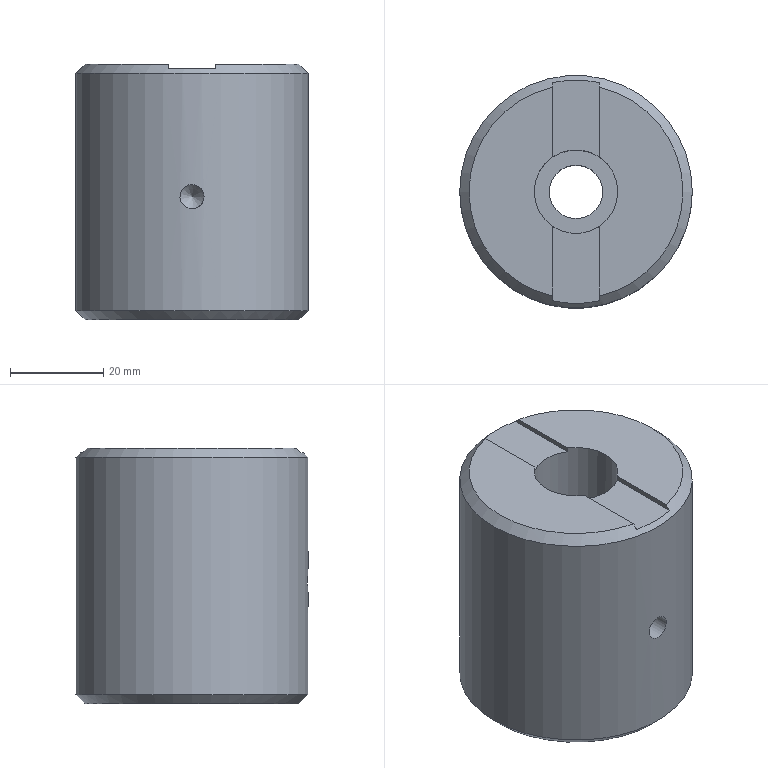Part | NX | features LIN_SOLID_COLOR 2 | 1 solid | 17 faces | box 50 x 50 x 55 mm | volume 97336 mm3 | plane 10 | cylinder 4 | cone 3 | commonest cylinder face diameters 5.2 x1 11.5 x1 18 x1 50 x1
STEP:
#1=CARTESIAN_POINT('',(609.,-200.,-46.5));
#2=VERTEX_POINT('',#1);
#3=CARTESIAN_POINT('',(586.,-200.,-46.5));
#4=DIRECTION('',(0.,0.,1.));
#5=DIRECTION('',(1.,0.,0.));
#6=AXIS2_PLACEMENT_3D('',#3,#4,#5);
#7=CIRCLE('',#6,23.);
#8=EDGE_CURVE('',#2,#2,#7,.T.);
#9=ORIENTED_EDGE('',*,*,#8,.F.);
#10=EDGE_LOOP('',(#9));
#11=FACE_BOUND('',#10,.T.);
#12=CARTESIAN_POINT('',(591.75,-200.,-46.5));
#13=VERTEX_POINT('',#12);
#14=CARTESIAN_POINT('',(586.,-200.,-46.5));
#15=DIRECTION('',(0.,0.,1.));
#16=DIRECTION('',(1.,0.,0.));
#17=AXIS2_PLACEMENT_3D('',#14,#15,#16);
#18=CIRCLE('',#17,5.75);
#19=EDGE_CURVE('',#13,#13,#18,.T.);
#20=ORIENTED_EDGE('',*,*,#19,.T.);
#21=EDGE_LOOP('',(#20));
#22=FACE_BOUND('',#21,.T.);
#23=CARTESIAN_POINT('',(586.,-200.,-46.5));
#24=DIRECTION('',(0.,0.,-1.));
#25=DIRECTION('',(1.,0.,0.));
#26=AXIS2_PLACEMENT_3D('',#23,#24,#25);
#27=PLANE('',#26);
#28=ADVANCED_FACE('',(#11,#22),#27,.T.);
#29=CARTESIAN_POINT('',(591.,-177.55,8.5));
#30=VERTEX_POINT('',#29);
#31=CARTESIAN_POINT('',(591.,-192.517,8.5));
#32=VERTEX_POINT('',#31);
#33=CARTESIAN_POINT('',(591.,-200.,8.5));
#34=DIRECTION('',(0.,-1.,0.));
#35=VECTOR('',#34,1000.);
#36=LINE('',#33,#35);
#37=EDGE_CURVE('',#30,#32,#36,.T.);
#38=ORIENTED_EDGE('',*,*,#37,.T.);
#39=CARTESIAN_POINT('',(591.,-207.483,8.5));
#40=VERTEX_POINT('',#39);
#41=CARTESIAN_POINT('',(586.,-200.,8.5));
#42=DIRECTION('',(0.,0.,-1.));
#43=DIRECTION('',(1.,0.,0.));
#44=AXIS2_PLACEMENT_3D('',#41,#42,#43);
#45=CIRCLE('',#44,9.);
#46=EDGE_CURVE('',#32,#40,#45,.T.);
#47=ORIENTED_EDGE('',*,*,#46,.T.);
#48=CARTESIAN_POINT('',(591.,-222.45,8.5));
#49=VERTEX_POINT('',#48);
#50=CARTESIAN_POINT('',(591.,-200.,8.5));
#51=DIRECTION('',(0.,-1.,0.));
#52=VECTOR('',#51,1000.);
#53=LINE('',#50,#52);
#54=EDGE_CURVE('',#40,#49,#53,.T.);
#55=ORIENTED_EDGE('',*,*,#54,.T.);
#56=CARTESIAN_POINT('',(586.,-200.,8.5));
#57=DIRECTION('',(0.,0.,-1.));
#58=DIRECTION('',(-1.,0.,0.));
#59=AXIS2_PLACEMENT_3D('',#56,#57,#58);
#60=CIRCLE('',#59,23.);
#61=EDGE_CURVE('',#30,#49,#60,.T.);
#62=ORIENTED_EDGE('',*,*,#61,.F.);
#63=EDGE_LOOP('',(#38,#47,#55,#62));
#64=FACE_BOUND('',#63,.T.);
#65=CARTESIAN_POINT('',(586.,-200.,8.5));
#66=DIRECTION('',(0.,0.,1.));
#67=DIRECTION('',(-1.,0.,0.));
#68=AXIS2_PLACEMENT_3D('',#65,#66,#67);
#69=PLANE('',#68);
#70=ADVANCED_FACE('',(#64),#69,.T.);
#71=CARTESIAN_POINT('',(581.,-222.45,8.5));
#72=VERTEX_POINT('',#71);
#73=CARTESIAN_POINT('',(581.,-207.483,8.5));
#74=VERTEX_POINT('',#73);
#75=CARTESIAN_POINT('',(581.,-200.,8.5));
#76=DIRECTION('',(0.,1.,0.));
#77=VECTOR('',#76,1000.);
#78=LINE('',#75,#77);
#79=EDGE_CURVE('',#72,#74,#78,.T.);
#80=ORIENTED_EDGE('',*,*,#79,.T.);
#81=CARTESIAN_POINT('',(581.,-192.517,8.5));
#82=VERTEX_POINT('',#81);
#83=CARTESIAN_POINT('',(586.,-200.,8.5));
#84=DIRECTION('',(0.,0.,-1.));
#85=DIRECTION('',(1.,0.,0.));
#86=AXIS2_PLACEMENT_3D('',#83,#84,#85);
#87=CIRCLE('',#86,9.);
#88=EDGE_CURVE('',#74,#82,#87,.T.);
#89=ORIENTED_EDGE('',*,*,#88,.T.);
#90=CARTESIAN_POINT('',(581.,-177.55,8.5));
#91=VERTEX_POINT('',#90);
#92=CARTESIAN_POINT('',(581.,-200.,8.5));
#93=DIRECTION('',(0.,1.,0.));
#94=VECTOR('',#93,1000.);
#95=LINE('',#92,#94);
#96=EDGE_CURVE('',#82,#91,#95,.T.);
#97=ORIENTED_EDGE('',*,*,#96,.T.);
#98=CARTESIAN_POINT('',(586.,-200.,8.5));
#99=DIRECTION('',(0.,0.,-1.));
#100=DIRECTION('',(-1.,0.,0.));
#101=AXIS2_PLACEMENT_3D('',#98,#99,#100);
#102=CIRCLE('',#101,23.);
#103=EDGE_CURVE('',#72,#91,#102,.T.);
#104=ORIENTED_EDGE('',*,*,#103,.F.);
#105=EDGE_LOOP('',(#80,#89,#97,#104));
#106=FACE_BOUND('',#105,.T.);
#107=CARTESIAN_POINT('',(586.,-200.,8.5));
#108=DIRECTION('',(0.,0.,1.));
#109=DIRECTION('',(-1.,0.,0.));
#110=AXIS2_PLACEMENT_3D('',#107,#108,#109);
#111=PLANE('',#110);
#112=ADVANCED_FACE('',(#106),#111,.T.);
#113=CARTESIAN_POINT('',(588.6,-224.864,-20.));
#114=VERTEX_POINT('',#113);
#115=CARTESIAN_POINT('',(588.036,-224.933,-22.04));
#116=CARTESIAN_POINT('',(588.882,-224.83,-19.999));
#117=CARTESIAN_POINT('',(588.036,-224.932,-17.962));
#118=CARTESIAN_POINT('',(586.002,-225.034,-17.119));
#119=CARTESIAN_POINT('',(583.963,-224.932,-17.961));
#120=CARTESIAN_POINT('',(583.119,-224.83,-19.999));
#121=CARTESIAN_POINT('',(583.961,-224.932,-22.035));
#122=CARTESIAN_POINT('',(585.997,-225.034,-22.881));
#123=CARTESIAN_POINT('',(588.036,-224.933,-22.04));
#124=CARTESIAN_POINT('',(588.882,-224.83,-19.999));
#125=CARTESIAN_POINT('',(588.036,-224.932,-17.962));
#126=B_SPLINE_CURVE_WITH_KNOTS('',3,(#115,#116,#117,#118,#119,#120,#121,#122,#123,#124,#125),.UNSPECIFIED.,.T.,.F.,(1,1,1,1,1,1,1,1,1,1,1,1,1,1,1),(-0.0061,-0.004067,-0.002033,0.,0.002033,0.004067,0.0061,0.008133,0.01017,0.0122,0.01423,0.01627,0.0183,0.02033,0.02237),.UNSPECIFIED.);
#127=EDGE_CURVE('',#114,#114,#126,.T.);
#128=ORIENTED_EDGE('',*,*,#127,.F.);
#129=EDGE_LOOP('',(#128));
#130=FACE_BOUND('',#129,.T.);
#131=CARTESIAN_POINT('',(611.,-200.,-44.5));
#132=VERTEX_POINT('',#131);
#133=CARTESIAN_POINT('',(586.,-200.,-44.5));
#134=DIRECTION('',(0.,0.,1.));
#135=DIRECTION('',(1.,0.,0.));
#136=AXIS2_PLACEMENT_3D('',#133,#134,#135);
#137=CIRCLE('',#136,25.);
#138=EDGE_CURVE('',#132,#132,#137,.F.);
#139=ORIENTED_EDGE('',*,*,#138,.F.);
#140=EDGE_LOOP('',(#139));
#141=FACE_BOUND('',#140,.T.);
#142=CARTESIAN_POINT('',(561.,-200.,6.5));
#143=VERTEX_POINT('',#142);
#144=CARTESIAN_POINT('',(586.,-200.,6.5));
#145=DIRECTION('',(0.,0.,-1.));
#146=DIRECTION('',(-1.,0.,0.));
#147=AXIS2_PLACEMENT_3D('',#144,#145,#146);
#148=CIRCLE('',#147,25.);
#149=EDGE_CURVE('',#143,#143,#148,.F.);
#150=ORIENTED_EDGE('',*,*,#149,.F.);
#151=EDGE_LOOP('',(#150));
#152=FACE_BOUND('',#151,.T.);
#153=CARTESIAN_POINT('',(586.,-200.,3.5));
#154=DIRECTION('',(0.,0.,-1.));
#155=DIRECTION('',(1.,0.,0.));
#156=AXIS2_PLACEMENT_3D('',#153,#154,#155);
#157=CYLINDRICAL_SURFACE('',#156,25.);
#158=ADVANCED_FACE('',(#130,#141,#152),#157,.T.);
#159=ORIENTED_EDGE('',*,*,#138,.T.);
#160=EDGE_LOOP('',(#159));
#161=FACE_BOUND('',#160,.T.);
#162=ORIENTED_EDGE('',*,*,#8,.T.);
#163=EDGE_LOOP('',(#162));
#164=FACE_BOUND('',#163,.T.);
#165=CARTESIAN_POINT('',(586.,-200.,-46.5));
#166=DIRECTION('',(0.,0.,1.));
#167=DIRECTION('',(-1.,0.,0.));
#168=AXIS2_PLACEMENT_3D('',#165,#166,#167);
#169=CONICAL_SURFACE('',#168,23.,0.7854);
#170=ADVANCED_FACE('',(#161,#164),#169,.T.);
#171=CARTESIAN_POINT('',(591.,-223.473,7.5));
#172=VERTEX_POINT('',#171);
#173=CARTESIAN_POINT('',(591.,-222.45,8.5));
#174=CARTESIAN_POINT('',(591.,-222.791,8.167));
#175=CARTESIAN_POINT('',(591.,-223.132,7.834));
#176=CARTESIAN_POINT('',(591.,-223.473,7.5));
#177=B_SPLINE_CURVE_WITH_KNOTS('',3,(#173,#174,#175,#176),.UNSPECIFIED.,.F.,.F.,(4,4),(0.1023,0.1037),.UNSPECIFIED.);
#178=EDGE_CURVE('',#49,#172,#177,.T.);
#179=ORIENTED_EDGE('',*,*,#178,.T.);
#180=CARTESIAN_POINT('',(581.,-223.473,7.5));
#181=VERTEX_POINT('',#180);
#182=CARTESIAN_POINT('',(586.,-200.,7.5));
#183=DIRECTION('',(0.,0.,1.));
#184=DIRECTION('',(1.,0.,0.));
#185=AXIS2_PLACEMENT_3D('',#182,#183,#184);
#186=CIRCLE('',#185,24.);
#187=EDGE_CURVE('',#172,#181,#186,.F.);
#188=ORIENTED_EDGE('',*,*,#187,.T.);
#189=CARTESIAN_POINT('',(581.,-223.473,7.5));
#190=CARTESIAN_POINT('',(581.,-223.132,7.834));
#191=CARTESIAN_POINT('',(581.,-222.791,8.167));
#192=CARTESIAN_POINT('',(581.,-222.45,8.5));
#193=B_SPLINE_CURVE_WITH_KNOTS('',3,(#189,#190,#191,#192),.UNSPECIFIED.,.F.,.F.,(4,4),(0.04264,0.04407),.UNSPECIFIED.);
#194=EDGE_CURVE('',#181,#72,#193,.T.);
#195=ORIENTED_EDGE('',*,*,#194,.T.);
#196=ORIENTED_EDGE('',*,*,#103,.T.);
#197=CARTESIAN_POINT('',(581.,-176.527,7.5));
#198=VERTEX_POINT('',#197);
#199=CARTESIAN_POINT('',(581.,-177.55,8.5));
#200=CARTESIAN_POINT('',(581.,-177.209,8.167));
#201=CARTESIAN_POINT('',(581.,-176.868,7.834));
#202=CARTESIAN_POINT('',(581.,-176.527,7.5));
#203=B_SPLINE_CURVE_WITH_KNOTS('',3,(#199,#200,#201,#202),.UNSPECIFIED.,.F.,.F.,(4,4),(0.1023,0.1037),.UNSPECIFIED.);
#204=EDGE_CURVE('',#91,#198,#203,.T.);
#205=ORIENTED_EDGE('',*,*,#204,.T.);
#206=CARTESIAN_POINT('',(591.,-176.527,7.5));
#207=VERTEX_POINT('',#206);
#208=CARTESIAN_POINT('',(586.,-200.,7.5));
#209=DIRECTION('',(0.,0.,1.));
#210=DIRECTION('',(1.,0.,0.));
#211=AXIS2_PLACEMENT_3D('',#208,#209,#210);
#212=CIRCLE('',#211,24.);
#213=EDGE_CURVE('',#198,#207,#212,.F.);
#214=ORIENTED_EDGE('',*,*,#213,.T.);
#215=CARTESIAN_POINT('',(591.,-176.527,7.5));
#216=CARTESIAN_POINT('',(591.,-176.868,7.834));
#217=CARTESIAN_POINT('',(591.,-177.209,8.167));
#218=CARTESIAN_POINT('',(591.,-177.55,8.5));
#219=B_SPLINE_CURVE_WITH_KNOTS('',3,(#215,#216,#217,#218),.UNSPECIFIED.,.F.,.F.,(4,4),(0.04264,0.04407),.UNSPECIFIED.);
#220=EDGE_CURVE('',#207,#30,#219,.T.);
#221=ORIENTED_EDGE('',*,*,#220,.T.);
#222=ORIENTED_EDGE('',*,*,#61,.T.);
#223=EDGE_LOOP('',(#179,#188,#195,#196,#205,#214,#221,#222));
#224=FACE_BOUND('',#223,.T.);
#225=ORIENTED_EDGE('',*,*,#149,.T.);
#226=EDGE_LOOP('',(#225));
#227=FACE_BOUND('',#226,.T.);
#228=CARTESIAN_POINT('',(586.,-200.,6.5));
#229=DIRECTION('',(0.,0.,-1.));
#230=DIRECTION('',(1.,0.,0.));
#231=AXIS2_PLACEMENT_3D('',#228,#229,#230);
#232=CONICAL_SURFACE('',#231,25.,0.7854);
#233=ADVANCED_FACE('',(#224,#227),#232,.T.);
#234=ORIENTED_EDGE('',*,*,#96,.F.);
#235=CARTESIAN_POINT('',(581.,-192.517,7.5));
#236=VERTEX_POINT('',#235);
#237=CARTESIAN_POINT('',(581.,-192.517,8.5));
#238=DIRECTION('',(0.,0.,-1.));
#239=VECTOR('',#238,1000.);
#240=LINE('',#237,#239);
#241=EDGE_CURVE('',#82,#236,#240,.T.);
#242=ORIENTED_EDGE('',*,*,#241,.T.);
#243=CARTESIAN_POINT('',(581.,-200.,7.5));
#244=DIRECTION('',(0.,1.,0.));
#245=VECTOR('',#244,1000.);
#246=LINE('',#243,#245);
#247=EDGE_CURVE('',#198,#236,#246,.F.);
#248=ORIENTED_EDGE('',*,*,#247,.F.);
#249=ORIENTED_EDGE('',*,*,#204,.F.);
#250=EDGE_LOOP('',(#234,#242,#248,#249));
#251=FACE_BOUND('',#250,.T.);
#252=CARTESIAN_POINT('',(581.,-200.,7.5));
#253=DIRECTION('',(-1.,0.,0.));
#254=DIRECTION('',(0.,0.,-1.));
#255=AXIS2_PLACEMENT_3D('',#252,#253,#254);
#256=PLANE('',#255);
#257=ADVANCED_FACE('',(#251),#256,.F.);
#258=ORIENTED_EDGE('',*,*,#247,.T.);
#259=CARTESIAN_POINT('',(591.,-192.517,7.5));
#260=VERTEX_POINT('',#259);
#261=CARTESIAN_POINT('',(586.,-200.,7.5));
#262=DIRECTION('',(0.,0.,-1.));
#263=DIRECTION('',(-1.,0.,0.));
#264=AXIS2_PLACEMENT_3D('',#261,#262,#263);
#265=CIRCLE('',#264,9.);
#266=EDGE_CURVE('',#236,#260,#265,.T.);
#267=ORIENTED_EDGE('',*,*,#266,.T.);
#268=CARTESIAN_POINT('',(591.,-200.,7.5));
#269=DIRECTION('',(0.,-1.,0.));
#270=VECTOR('',#269,1000.);
#271=LINE('',#268,#270);
#272=EDGE_CURVE('',#260,#207,#271,.F.);
#273=ORIENTED_EDGE('',*,*,#272,.T.);
#274=ORIENTED_EDGE('',*,*,#213,.F.);
#275=EDGE_LOOP('',(#258,#267,#273,#274));
#276=FACE_BOUND('',#275,.T.);
#277=CARTESIAN_POINT('',(586.,-200.,7.5));
#278=DIRECTION('',(0.,0.,-1.));
#279=DIRECTION('',(1.,0.,0.));
#280=AXIS2_PLACEMENT_3D('',#277,#278,#279);
#281=PLANE('',#280);
#282=ADVANCED_FACE('',(#276),#281,.F.);
#283=ORIENTED_EDGE('',*,*,#272,.F.);
#284=CARTESIAN_POINT('',(591.,-192.517,8.5));
#285=DIRECTION('',(0.,0.,-1.));
#286=VECTOR('',#285,1000.);
#287=LINE('',#284,#286);
#288=EDGE_CURVE('',#260,#32,#287,.F.);
#289=ORIENTED_EDGE('',*,*,#288,.T.);
#290=ORIENTED_EDGE('',*,*,#37,.F.);
#291=ORIENTED_EDGE('',*,*,#220,.F.);
#292=EDGE_LOOP('',(#283,#289,#290,#291));
#293=FACE_BOUND('',#292,.T.);
#294=CARTESIAN_POINT('',(591.,-200.,7.5));
#295=DIRECTION('',(1.,0.,0.));
#296=DIRECTION('',(0.,0.,1.));
#297=AXIS2_PLACEMENT_3D('',#294,#295,#296);
#298=PLANE('',#297);
#299=ADVANCED_FACE('',(#293),#298,.F.);
#300=ORIENTED_EDGE('',*,*,#54,.F.);
#301=CARTESIAN_POINT('',(591.,-207.483,7.5));
#302=VERTEX_POINT('',#301);
#303=CARTESIAN_POINT('',(591.,-207.483,8.5));
#304=DIRECTION('',(0.,0.,-1.));
#305=VECTOR('',#304,1000.);
#306=LINE('',#303,#305);
#307=EDGE_CURVE('',#40,#302,#306,.T.);
#308=ORIENTED_EDGE('',*,*,#307,.T.);
#309=CARTESIAN_POINT('',(591.,-200.,7.5));
#310=DIRECTION('',(0.,-1.,0.));
#311=VECTOR('',#310,1000.);
#312=LINE('',#309,#311);
#313=EDGE_CURVE('',#172,#302,#312,.F.);
#314=ORIENTED_EDGE('',*,*,#313,.F.);
#315=ORIENTED_EDGE('',*,*,#178,.F.);
#316=EDGE_LOOP('',(#300,#308,#314,#315));
#317=FACE_BOUND('',#316,.T.);
#318=CARTESIAN_POINT('',(591.,-200.,7.5));
#319=DIRECTION('',(1.,0.,0.));
#320=DIRECTION('',(0.,0.,1.));
#321=AXIS2_PLACEMENT_3D('',#318,#319,#320);
#322=PLANE('',#321);
#323=ADVANCED_FACE('',(#317),#322,.F.);
#324=ORIENTED_EDGE('',*,*,#313,.T.);
#325=CARTESIAN_POINT('',(581.,-207.483,7.5));
#326=VERTEX_POINT('',#325);
#327=CARTESIAN_POINT('',(586.,-200.,7.5));
#328=DIRECTION('',(0.,0.,-1.));
#329=DIRECTION('',(-1.,0.,0.));
#330=AXIS2_PLACEMENT_3D('',#327,#328,#329);
#331=CIRCLE('',#330,9.);
#332=EDGE_CURVE('',#302,#326,#331,.T.);
#333=ORIENTED_EDGE('',*,*,#332,.T.);
#334=CARTESIAN_POINT('',(581.,-200.,7.5));
#335=DIRECTION('',(0.,1.,0.));
#336=VECTOR('',#335,1000.);
#337=LINE('',#334,#336);
#338=EDGE_CURVE('',#326,#181,#337,.F.);
#339=ORIENTED_EDGE('',*,*,#338,.T.);
#340=ORIENTED_EDGE('',*,*,#187,.F.);
#341=EDGE_LOOP('',(#324,#333,#339,#340));
#342=FACE_BOUND('',#341,.T.);
#343=CARTESIAN_POINT('',(586.,-200.,7.5));
#344=DIRECTION('',(0.,0.,-1.));
#345=DIRECTION('',(1.,0.,0.));
#346=AXIS2_PLACEMENT_3D('',#343,#344,#345);
#347=PLANE('',#346);
#348=ADVANCED_FACE('',(#342),#347,.F.);
#349=ORIENTED_EDGE('',*,*,#338,.F.);
#350=CARTESIAN_POINT('',(581.,-207.483,8.5));
#351=DIRECTION('',(0.,0.,-1.));
#352=VECTOR('',#351,1000.);
#353=LINE('',#350,#352);
#354=EDGE_CURVE('',#326,#74,#353,.F.);
#355=ORIENTED_EDGE('',*,*,#354,.T.);
#356=ORIENTED_EDGE('',*,*,#79,.F.);
#357=ORIENTED_EDGE('',*,*,#194,.F.);
#358=EDGE_LOOP('',(#349,#355,#356,#357));
#359=FACE_BOUND('',#358,.T.);
#360=CARTESIAN_POINT('',(581.,-200.,7.5));
#361=DIRECTION('',(-1.,0.,0.));
#362=DIRECTION('',(0.,0.,-1.));
#363=AXIS2_PLACEMENT_3D('',#360,#361,#362);
#364=PLANE('',#363);
#365=ADVANCED_FACE('',(#359),#364,.F.);
#366=CARTESIAN_POINT('',(577.,-200.,-16.5));
#367=VERTEX_POINT('',#366);
#368=CARTESIAN_POINT('',(586.,-200.,-16.5));
#369=DIRECTION('',(0.,0.,-1.));
#370=DIRECTION('',(-1.,0.,0.));
#371=AXIS2_PLACEMENT_3D('',#368,#369,#370);
#372=CIRCLE('',#371,9.);
#373=EDGE_CURVE('',#367,#367,#372,.T.);
#374=ORIENTED_EDGE('',*,*,#373,.T.);
#375=EDGE_LOOP('',(#374));
#376=FACE_BOUND('',#375,.T.);
#377=ORIENTED_EDGE('',*,*,#88,.F.);
#378=ORIENTED_EDGE('',*,*,#354,.F.);
#379=ORIENTED_EDGE('',*,*,#332,.F.);
#380=ORIENTED_EDGE('',*,*,#307,.F.);
#381=ORIENTED_EDGE('',*,*,#46,.F.);
#382=ORIENTED_EDGE('',*,*,#288,.F.);
#383=ORIENTED_EDGE('',*,*,#266,.F.);
#384=ORIENTED_EDGE('',*,*,#241,.F.);
#385=EDGE_LOOP('',(#377,#378,#379,#380,#381,#382,#383,#384));
#386=FACE_BOUND('',#385,.T.);
#387=CARTESIAN_POINT('',(586.,-200.,8.5));
#388=DIRECTION('',(0.,0.,-1.));
#389=DIRECTION('',(1.,0.,0.));
#390=AXIS2_PLACEMENT_3D('',#387,#388,#389);
#391=CYLINDRICAL_SURFACE('',#390,9.);
#392=ADVANCED_FACE('',(#376,#386),#391,.F.);
#393=CARTESIAN_POINT('',(580.25,-200.,-16.5));
#394=VERTEX_POINT('',#393);
#395=CARTESIAN_POINT('',(586.,-200.,-16.5));
#396=DIRECTION('',(0.,0.,-1.));
#397=DIRECTION('',(-1.,0.,0.));
#398=AXIS2_PLACEMENT_3D('',#395,#396,#397);
#399=CIRCLE('',#398,5.75);
#400=EDGE_CURVE('',#394,#394,#399,.T.);
#401=ORIENTED_EDGE('',*,*,#400,.T.);
#402=EDGE_LOOP('',(#401));
#403=FACE_BOUND('',#402,.T.);
#404=ORIENTED_EDGE('',*,*,#373,.F.);
#405=EDGE_LOOP('',(#404));
#406=FACE_BOUND('',#405,.T.);
#407=CARTESIAN_POINT('',(586.,-200.,-16.5));
#408=DIRECTION('',(0.,0.,-1.));
#409=DIRECTION('',(1.,0.,0.));
#410=AXIS2_PLACEMENT_3D('',#407,#408,#409);
#411=PLANE('',#410);
#412=ADVANCED_FACE('',(#403,#406),#411,.F.);
#413=ORIENTED_EDGE('',*,*,#19,.F.);
#414=EDGE_LOOP('',(#413));
#415=FACE_BOUND('',#414,.T.);
#416=ORIENTED_EDGE('',*,*,#400,.F.);
#417=EDGE_LOOP('',(#416));
#418=FACE_BOUND('',#417,.T.);
#419=CARTESIAN_POINT('',(586.,-200.,8.5));
#420=DIRECTION('',(0.,0.,-1.));
#421=DIRECTION('',(1.,0.,0.));
#422=AXIS2_PLACEMENT_3D('',#419,#420,#421);
#423=CYLINDRICAL_SURFACE('',#422,5.75);
#424=ADVANCED_FACE('',(#415,#418),#423,.F.);
#425=ORIENTED_EDGE('',*,*,#127,.T.);
#426=EDGE_LOOP('',(#425));
#427=FACE_BOUND('',#426,.T.);
#428=CARTESIAN_POINT('',(583.4,-213.1,-20.));
#429=VERTEX_POINT('',#428);
#430=CARTESIAN_POINT('',(586.,-213.1,-20.));
#431=DIRECTION('',(0.,-1.,0.));
#432=DIRECTION('',(-1.,0.,0.));
#433=AXIS2_PLACEMENT_3D('',#430,#431,#432);
#434=CIRCLE('',#433,2.6);
#435=EDGE_CURVE('',#429,#429,#434,.T.);
#436=ORIENTED_EDGE('',*,*,#435,.F.);
#437=EDGE_LOOP('',(#436));
#438=FACE_BOUND('',#437,.T.);
#439=CARTESIAN_POINT('',(586.,-234.5,-20.));
#440=DIRECTION('',(0.,1.,0.));
#441=DIRECTION('',(1.,0.,0.));
#442=AXIS2_PLACEMENT_3D('',#439,#440,#441);
#443=CYLINDRICAL_SURFACE('',#442,2.6);
#444=ADVANCED_FACE('',(#427,#438),#443,.F.);
#445=CARTESIAN_POINT('',(586.,-210.5,-20.));
#446=VERTEX_POINT('',#445);
#447=VERTEX_LOOP('',#446);
#448=FACE_BOUND('',#447,.T.);
#449=ORIENTED_EDGE('',*,*,#435,.T.);
#450=EDGE_LOOP('',(#449));
#451=FACE_BOUND('',#450,.T.);
#452=CARTESIAN_POINT('',(586.,-213.1,-20.));
#453=DIRECTION('',(0.,-1.,0.));
#454=DIRECTION('',(1.,0.,0.));
#455=AXIS2_PLACEMENT_3D('',#452,#453,#454);
#456=CONICAL_SURFACE('',#455,2.6,0.7854);
#457=ADVANCED_FACE('',(#448,#451),#456,.F.);
#458=CLOSED_SHELL('',(#28,#70,#112,#158,#170,#233,#257,#282,#299,#323,#348,#365,#392,#412,#424,#444,#457));
#459=MANIFOLD_SOLID_BREP('',#458);
#460=(LENGTH_UNIT()NAMED_UNIT(*)SI_UNIT(.MILLI.,.METRE.));
#461=UNCERTAINTY_MEASURE_WITH_UNIT(LENGTH_MEASURE(0.0508),#460,'','');
#462=(NAMED_UNIT(*)PLANE_ANGLE_UNIT()SI_UNIT($,.RADIAN.));
#463=(NAMED_UNIT(*)SI_UNIT($,.STERADIAN.)SOLID_ANGLE_UNIT());
#464=(GEOMETRIC_REPRESENTATION_CONTEXT(3)GLOBAL_UNCERTAINTY_ASSIGNED_CONTEXT((#461))GLOBAL_UNIT_ASSIGNED_CONTEXT((#460,#462,#463))REPRESENTATION_CONTEXT('',''));
#465=ADVANCED_BREP_SHAPE_REPRESENTATION('',(#459),#464);